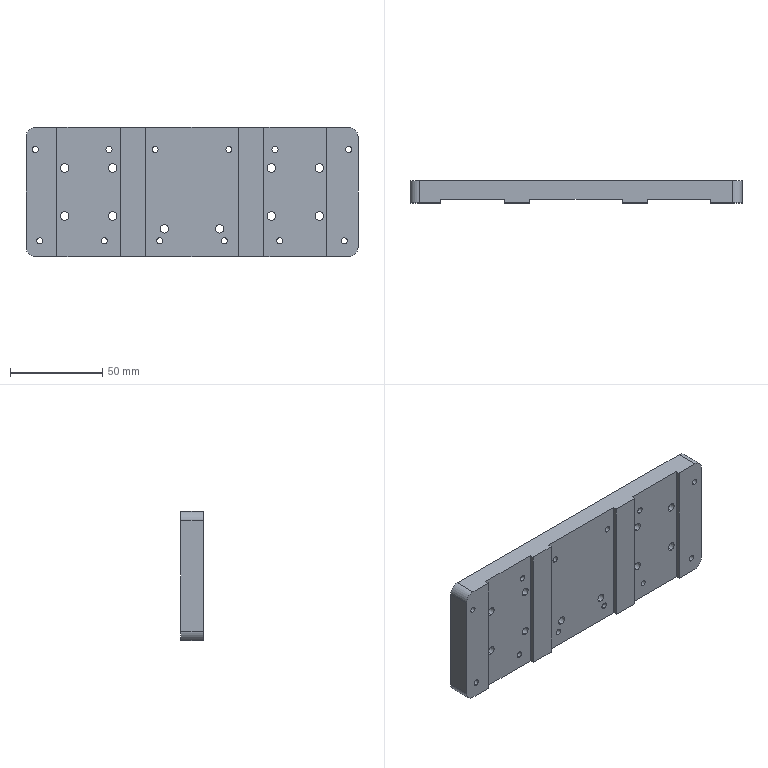Part | STEP file | 1 solid | 96 faces | box 180 x 12 x 70 mm | volume 130133 mm3 | cylinder 68 | plane 28 | commonest cylinder face diameters 3.3 x24 4.5 x20 7.9 x16 8 x4 10 x4